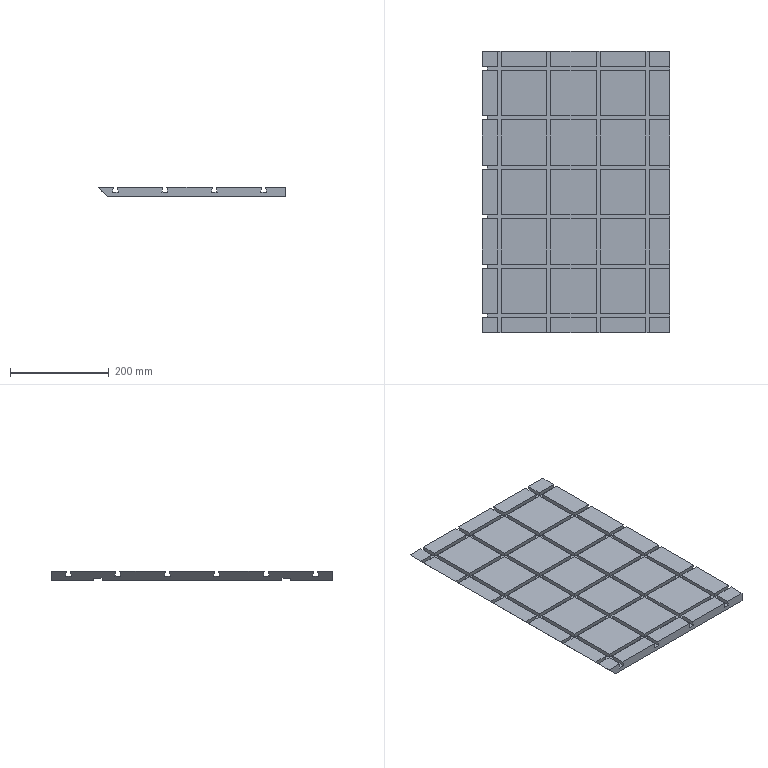Part | STEP file | Superstructure_1 | 1 solid | 165 faces | box 380 x 570 x 19 mm | volume 3518605 mm3 | plane 165